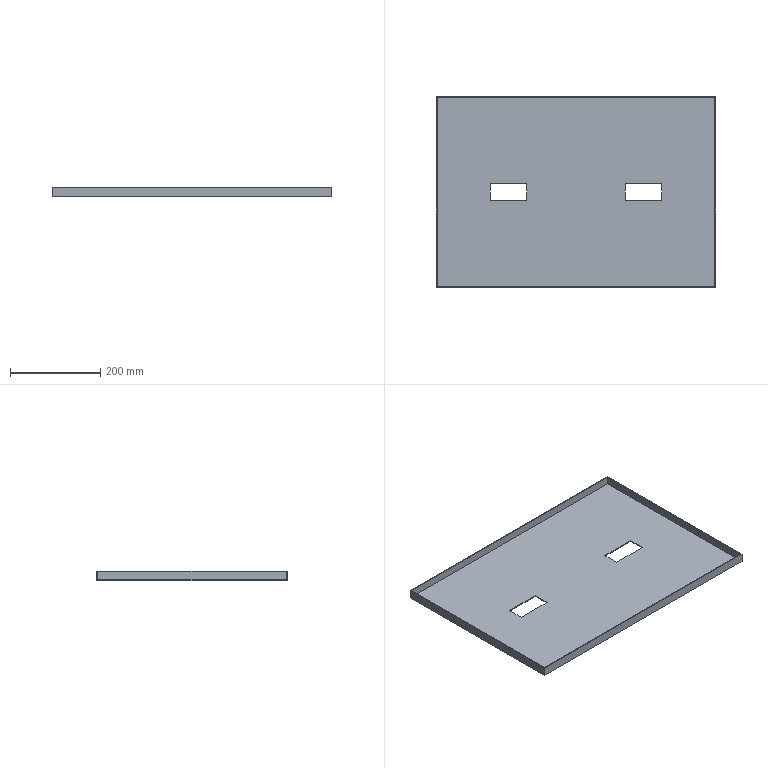Part | STEP file | Rear sealing plate | 1 solid | 19 faces | box 620 x 421.75 x 20 mm | volume 585700 mm3 | plane 19
STEP:
#1=CARTESIAN_POINT('',(0.,0.,0.));
#2=DIRECTION('',(0.,0.,1.));
#3=DIRECTION('',(1.,0.,0.));
#4=AXIS2_PLACEMENT_3D('',#1,#2,#3);
#5=CARTESIAN_POINT('',(-310.,-210.875,0.));
#6=VERTEX_POINT('',#5);
#7=CARTESIAN_POINT('',(310.,-210.875,0.));
#8=VERTEX_POINT('',#7);
#9=CARTESIAN_POINT('',(0.,-210.875,0.));
#10=DIRECTION('',(1.,0.,0.));
#11=VECTOR('',#10,1.);
#12=LINE('',#9,#11);
#13=CARTESIAN_POINT('',(0.,0.,0.));
#14=DIRECTION('',(0.,0.,1.));
#15=DIRECTION('',(1.,0.,0.));
#16=AXIS2_PLACEMENT_3D('',#13,#14,#15);
#17=PLANE('',#16);
#18=CARTESIAN_POINT('',(0.,-210.875));
#19=DIRECTION('',(1.,0.));
#20=VECTOR('',#19,1.);
#21=LINE('',#18,#20);
#22=(GEOMETRIC_REPRESENTATION_CONTEXT(2)PARAMETRIC_REPRESENTATION_CONTEXT()REPRESENTATION_CONTEXT('',''));
#23=DEFINITIONAL_REPRESENTATION('',(#21),#22);
#24=PCURVE('',#17,#23);
#25=CARTESIAN_POINT('',(-310.,-210.875,20.));
#26=DIRECTION('',(0.,1.,0.));
#27=DIRECTION('',(0.,0.,1.));
#28=AXIS2_PLACEMENT_3D('',#25,#26,#27);
#29=PLANE('',#28);
#30=CARTESIAN_POINT('',(-20.,310.));
#31=DIRECTION('',(0.,1.));
#32=VECTOR('',#31,1.);
#33=LINE('',#30,#32);
#34=(GEOMETRIC_REPRESENTATION_CONTEXT(2)PARAMETRIC_REPRESENTATION_CONTEXT()REPRESENTATION_CONTEXT('',''));
#35=DEFINITIONAL_REPRESENTATION('',(#33),#34);
#36=PCURVE('',#29,#35);
#37=SURFACE_CURVE('',#12,(#24,#36),.PCURVE_S1.);
#38=EDGE_CURVE('',#6,#8,#37,.T.);
#39=ORIENTED_EDGE('',*,*,#38,.F.);
#40=CARTESIAN_POINT('',(-310.,210.875,0.));
#41=VERTEX_POINT('',#40);
#42=CARTESIAN_POINT('',(-310.,0.,0.));
#43=DIRECTION('',(0.,-1.,0.));
#44=VECTOR('',#43,1.);
#45=LINE('',#42,#44);
#46=CARTESIAN_POINT('',(-310.,0.));
#47=DIRECTION('',(0.,-1.));
#48=VECTOR('',#47,1.);
#49=LINE('',#46,#48);
#50=(GEOMETRIC_REPRESENTATION_CONTEXT(2)PARAMETRIC_REPRESENTATION_CONTEXT()REPRESENTATION_CONTEXT('',''));
#51=DEFINITIONAL_REPRESENTATION('',(#49),#50);
#52=PCURVE('',#17,#51);
#53=CARTESIAN_POINT('',(-310.,210.875,20.));
#54=DIRECTION('',(1.,0.,0.));
#55=DIRECTION('',(0.,0.,-1.));
#56=AXIS2_PLACEMENT_3D('',#53,#54,#55);
#57=PLANE('',#56);
#58=CARTESIAN_POINT('',(20.,-210.875));
#59=DIRECTION('',(0.,-1.));
#60=VECTOR('',#59,1.);
#61=LINE('',#58,#60);
#62=(GEOMETRIC_REPRESENTATION_CONTEXT(2)PARAMETRIC_REPRESENTATION_CONTEXT()REPRESENTATION_CONTEXT('',''));
#63=DEFINITIONAL_REPRESENTATION('',(#61),#62);
#64=PCURVE('',#57,#63);
#65=SURFACE_CURVE('',#45,(#52,#64),.PCURVE_S1.);
#66=EDGE_CURVE('',#41,#6,#65,.T.);
#67=ORIENTED_EDGE('',*,*,#66,.F.);
#68=CARTESIAN_POINT('',(310.,210.875,0.));
#69=VERTEX_POINT('',#68);
#70=CARTESIAN_POINT('',(0.,210.875,0.));
#71=DIRECTION('',(-1.,0.,0.));
#72=VECTOR('',#71,1.);
#73=LINE('',#70,#72);
#74=CARTESIAN_POINT('',(0.,210.875));
#75=DIRECTION('',(-1.,0.));
#76=VECTOR('',#75,1.);
#77=LINE('',#74,#76);
#78=(GEOMETRIC_REPRESENTATION_CONTEXT(2)PARAMETRIC_REPRESENTATION_CONTEXT()REPRESENTATION_CONTEXT('',''));
#79=DEFINITIONAL_REPRESENTATION('',(#77),#78);
#80=PCURVE('',#17,#79);
#81=CARTESIAN_POINT('',(-310.,210.875,20.));
#82=DIRECTION('',(0.,-1.,0.));
#83=DIRECTION('',(0.,0.,-1.));
#84=AXIS2_PLACEMENT_3D('',#81,#82,#83);
#85=PLANE('',#84);
#86=CARTESIAN_POINT('',(20.,310.));
#87=DIRECTION('',(0.,-1.));
#88=VECTOR('',#87,1.);
#89=LINE('',#86,#88);
#90=(GEOMETRIC_REPRESENTATION_CONTEXT(2)PARAMETRIC_REPRESENTATION_CONTEXT()REPRESENTATION_CONTEXT('',''));
#91=DEFINITIONAL_REPRESENTATION('',(#89),#90);
#92=PCURVE('',#85,#91);
#93=SURFACE_CURVE('',#73,(#80,#92),.PCURVE_S1.);
#94=EDGE_CURVE('',#69,#41,#93,.T.);
#95=ORIENTED_EDGE('',*,*,#94,.F.);
#96=CARTESIAN_POINT('',(310.,0.,0.));
#97=DIRECTION('',(0.,1.,0.));
#98=VECTOR('',#97,1.);
#99=LINE('',#96,#98);
#100=CARTESIAN_POINT('',(310.,0.));
#101=DIRECTION('',(0.,1.));
#102=VECTOR('',#101,1.);
#103=LINE('',#100,#102);
#104=(GEOMETRIC_REPRESENTATION_CONTEXT(2)PARAMETRIC_REPRESENTATION_CONTEXT()REPRESENTATION_CONTEXT('',''));
#105=DEFINITIONAL_REPRESENTATION('',(#103),#104);
#106=PCURVE('',#17,#105);
#107=CARTESIAN_POINT('',(310.,210.875,20.));
#108=DIRECTION('',(-1.,0.,0.));
#109=DIRECTION('',(0.,-1.,0.));
#110=AXIS2_PLACEMENT_3D('',#107,#108,#109);
#111=PLANE('',#110);
#112=CARTESIAN_POINT('',(210.875,-20.));
#113=DIRECTION('',(-1.,0.));
#114=VECTOR('',#113,1.);
#115=LINE('',#112,#114);
#116=(GEOMETRIC_REPRESENTATION_CONTEXT(2)PARAMETRIC_REPRESENTATION_CONTEXT()REPRESENTATION_CONTEXT('',''));
#117=DEFINITIONAL_REPRESENTATION('',(#115),#116);
#118=PCURVE('',#111,#117);
#119=SURFACE_CURVE('',#99,(#106,#118),.PCURVE_S1.);
#120=EDGE_CURVE('',#8,#69,#119,.T.);
#121=ORIENTED_EDGE('',*,*,#120,.F.);
#122=EDGE_LOOP('',(#39,#67,#95,#121));
#123=FACE_BOUND('',#122,.T.);
#124=CARTESIAN_POINT('',(109.,-18.5,0.));
#125=VERTEX_POINT('',#124);
#126=CARTESIAN_POINT('',(109.,18.5,0.));
#127=VERTEX_POINT('',#126);
#128=CARTESIAN_POINT('',(109.,0.,0.));
#129=DIRECTION('',(0.,1.,0.));
#130=VECTOR('',#129,1.);
#131=LINE('',#128,#130);
#132=CARTESIAN_POINT('',(109.,0.));
#133=DIRECTION('',(0.,1.));
#134=VECTOR('',#133,1.);
#135=LINE('',#132,#134);
#136=(GEOMETRIC_REPRESENTATION_CONTEXT(2)PARAMETRIC_REPRESENTATION_CONTEXT()REPRESENTATION_CONTEXT('',''));
#137=DEFINITIONAL_REPRESENTATION('',(#135),#136);
#138=PCURVE('',#17,#137);
#139=CARTESIAN_POINT('',(109.,18.5,20.));
#140=DIRECTION('',(-1.,0.,0.));
#141=DIRECTION('',(0.,0.,1.));
#142=AXIS2_PLACEMENT_3D('',#139,#140,#141);
#143=PLANE('',#142);
#144=CARTESIAN_POINT('',(-20.,-18.5));
#145=DIRECTION('',(0.,1.));
#146=VECTOR('',#145,1.);
#147=LINE('',#144,#146);
#148=(GEOMETRIC_REPRESENTATION_CONTEXT(2)PARAMETRIC_REPRESENTATION_CONTEXT()REPRESENTATION_CONTEXT('',''));
#149=DEFINITIONAL_REPRESENTATION('',(#147),#148);
#150=PCURVE('',#143,#149);
#151=SURFACE_CURVE('',#131,(#138,#150),.PCURVE_S1.);
#152=EDGE_CURVE('',#125,#127,#151,.T.);
#153=ORIENTED_EDGE('',*,*,#152,.F.);
#154=CARTESIAN_POINT('',(190.,-18.5,0.));
#155=VERTEX_POINT('',#154);
#156=CARTESIAN_POINT('',(0.,-18.5,0.));
#157=DIRECTION('',(-1.,0.,0.));
#158=VECTOR('',#157,1.);
#159=LINE('',#156,#158);
#160=CARTESIAN_POINT('',(0.,-18.5));
#161=DIRECTION('',(-1.,0.));
#162=VECTOR('',#161,1.);
#163=LINE('',#160,#162);
#164=(GEOMETRIC_REPRESENTATION_CONTEXT(2)PARAMETRIC_REPRESENTATION_CONTEXT()REPRESENTATION_CONTEXT('',''));
#165=DEFINITIONAL_REPRESENTATION('',(#163),#164);
#166=PCURVE('',#17,#165);
#167=CARTESIAN_POINT('',(190.,-18.5,20.));
#168=DIRECTION('',(0.,-1.,0.));
#169=DIRECTION('',(0.,0.,-1.));
#170=AXIS2_PLACEMENT_3D('',#167,#168,#169);
#171=PLANE('',#170);
#172=CARTESIAN_POINT('',(20.,-190.));
#173=DIRECTION('',(0.,-1.));
#174=VECTOR('',#173,1.);
#175=LINE('',#172,#174);
#176=(GEOMETRIC_REPRESENTATION_CONTEXT(2)PARAMETRIC_REPRESENTATION_CONTEXT()REPRESENTATION_CONTEXT('',''));
#177=DEFINITIONAL_REPRESENTATION('',(#175),#176);
#178=PCURVE('',#171,#177);
#179=SURFACE_CURVE('',#159,(#166,#178),.PCURVE_S1.);
#180=EDGE_CURVE('',#155,#125,#179,.T.);
#181=ORIENTED_EDGE('',*,*,#180,.F.);
#182=CARTESIAN_POINT('',(190.,18.5,0.));
#183=VERTEX_POINT('',#182);
#184=CARTESIAN_POINT('',(190.,0.,0.));
#185=DIRECTION('',(0.,-1.,0.));
#186=VECTOR('',#185,1.);
#187=LINE('',#184,#186);
#188=CARTESIAN_POINT('',(190.,0.));
#189=DIRECTION('',(0.,-1.));
#190=VECTOR('',#189,1.);
#191=LINE('',#188,#190);
#192=(GEOMETRIC_REPRESENTATION_CONTEXT(2)PARAMETRIC_REPRESENTATION_CONTEXT()REPRESENTATION_CONTEXT('',''));
#193=DEFINITIONAL_REPRESENTATION('',(#191),#192);
#194=PCURVE('',#17,#193);
#195=CARTESIAN_POINT('',(190.,18.5,20.));
#196=DIRECTION('',(1.,0.,0.));
#197=DIRECTION('',(0.,0.,-1.));
#198=AXIS2_PLACEMENT_3D('',#195,#196,#197);
#199=PLANE('',#198);
#200=CARTESIAN_POINT('',(20.,-18.5));
#201=DIRECTION('',(0.,-1.));
#202=VECTOR('',#201,1.);
#203=LINE('',#200,#202);
#204=(GEOMETRIC_REPRESENTATION_CONTEXT(2)PARAMETRIC_REPRESENTATION_CONTEXT()REPRESENTATION_CONTEXT('',''));
#205=DEFINITIONAL_REPRESENTATION('',(#203),#204);
#206=PCURVE('',#199,#205);
#207=SURFACE_CURVE('',#187,(#194,#206),.PCURVE_S1.);
#208=EDGE_CURVE('',#183,#155,#207,.T.);
#209=ORIENTED_EDGE('',*,*,#208,.F.);
#210=CARTESIAN_POINT('',(0.,18.5,0.));
#211=DIRECTION('',(1.,0.,0.));
#212=VECTOR('',#211,1.);
#213=LINE('',#210,#212);
#214=CARTESIAN_POINT('',(0.,18.5));
#215=DIRECTION('',(1.,0.));
#216=VECTOR('',#215,1.);
#217=LINE('',#214,#216);
#218=(GEOMETRIC_REPRESENTATION_CONTEXT(2)PARAMETRIC_REPRESENTATION_CONTEXT()REPRESENTATION_CONTEXT('',''));
#219=DEFINITIONAL_REPRESENTATION('',(#217),#218);
#220=PCURVE('',#17,#219);
#221=CARTESIAN_POINT('',(190.,18.5,20.));
#222=DIRECTION('',(0.,1.,0.));
#223=DIRECTION('',(-1.,0.,0.));
#224=AXIS2_PLACEMENT_3D('',#221,#222,#223);
#225=PLANE('',#224);
#226=CARTESIAN_POINT('',(190.,-20.));
#227=DIRECTION('',(-1.,0.));
#228=VECTOR('',#227,1.);
#229=LINE('',#226,#228);
#230=(GEOMETRIC_REPRESENTATION_CONTEXT(2)PARAMETRIC_REPRESENTATION_CONTEXT()REPRESENTATION_CONTEXT('',''));
#231=DEFINITIONAL_REPRESENTATION('',(#229),#230);
#232=PCURVE('',#225,#231);
#233=SURFACE_CURVE('',#213,(#220,#232),.PCURVE_S1.);
#234=EDGE_CURVE('',#127,#183,#233,.T.);
#235=ORIENTED_EDGE('',*,*,#234,.F.);
#236=EDGE_LOOP('',(#153,#181,#209,#235));
#237=FACE_BOUND('',#236,.T.);
#238=CARTESIAN_POINT('',(-190.,-18.5,0.));
#239=VERTEX_POINT('',#238);
#240=CARTESIAN_POINT('',(-190.,18.5,0.));
#241=VERTEX_POINT('',#240);
#242=CARTESIAN_POINT('',(-190.,0.,0.));
#243=DIRECTION('',(0.,1.,0.));
#244=VECTOR('',#243,1.);
#245=LINE('',#242,#244);
#246=CARTESIAN_POINT('',(-190.,0.));
#247=DIRECTION('',(0.,1.));
#248=VECTOR('',#247,1.);
#249=LINE('',#246,#248);
#250=(GEOMETRIC_REPRESENTATION_CONTEXT(2)PARAMETRIC_REPRESENTATION_CONTEXT()REPRESENTATION_CONTEXT('',''));
#251=DEFINITIONAL_REPRESENTATION('',(#249),#250);
#252=PCURVE('',#17,#251);
#253=CARTESIAN_POINT('',(-190.,18.5,20.));
#254=DIRECTION('',(-1.,0.,0.));
#255=DIRECTION('',(0.,0.,1.));
#256=AXIS2_PLACEMENT_3D('',#253,#254,#255);
#257=PLANE('',#256);
#258=CARTESIAN_POINT('',(-20.,-18.5));
#259=DIRECTION('',(0.,1.));
#260=VECTOR('',#259,1.);
#261=LINE('',#258,#260);
#262=(GEOMETRIC_REPRESENTATION_CONTEXT(2)PARAMETRIC_REPRESENTATION_CONTEXT()REPRESENTATION_CONTEXT('',''));
#263=DEFINITIONAL_REPRESENTATION('',(#261),#262);
#264=PCURVE('',#257,#263);
#265=SURFACE_CURVE('',#245,(#252,#264),.PCURVE_S1.);
#266=EDGE_CURVE('',#239,#241,#265,.T.);
#267=ORIENTED_EDGE('',*,*,#266,.F.);
#268=CARTESIAN_POINT('',(-109.,-18.5,0.));
#269=VERTEX_POINT('',#268);
#270=CARTESIAN_POINT('',(0.,-18.5,0.));
#271=DIRECTION('',(-1.,0.,0.));
#272=VECTOR('',#271,1.);
#273=LINE('',#270,#272);
#274=CARTESIAN_POINT('',(0.,-18.5));
#275=DIRECTION('',(-1.,0.));
#276=VECTOR('',#275,1.);
#277=LINE('',#274,#276);
#278=(GEOMETRIC_REPRESENTATION_CONTEXT(2)PARAMETRIC_REPRESENTATION_CONTEXT()REPRESENTATION_CONTEXT('',''));
#279=DEFINITIONAL_REPRESENTATION('',(#277),#278);
#280=PCURVE('',#17,#279);
#281=CARTESIAN_POINT('',(-109.,-18.5,20.));
#282=DIRECTION('',(0.,-1.,0.));
#283=DIRECTION('',(0.,0.,-1.));
#284=AXIS2_PLACEMENT_3D('',#281,#282,#283);
#285=PLANE('',#284);
#286=CARTESIAN_POINT('',(20.,109.));
#287=DIRECTION('',(0.,-1.));
#288=VECTOR('',#287,1.);
#289=LINE('',#286,#288);
#290=(GEOMETRIC_REPRESENTATION_CONTEXT(2)PARAMETRIC_REPRESENTATION_CONTEXT()REPRESENTATION_CONTEXT('',''));
#291=DEFINITIONAL_REPRESENTATION('',(#289),#290);
#292=PCURVE('',#285,#291);
#293=SURFACE_CURVE('',#273,(#280,#292),.PCURVE_S1.);
#294=EDGE_CURVE('',#269,#239,#293,.T.);
#295=ORIENTED_EDGE('',*,*,#294,.F.);
#296=CARTESIAN_POINT('',(-109.,18.5,0.));
#297=VERTEX_POINT('',#296);
#298=CARTESIAN_POINT('',(-109.,0.,0.));
#299=DIRECTION('',(0.,-1.,0.));
#300=VECTOR('',#299,1.);
#301=LINE('',#298,#300);
#302=CARTESIAN_POINT('',(-109.,0.));
#303=DIRECTION('',(0.,-1.));
#304=VECTOR('',#303,1.);
#305=LINE('',#302,#304);
#306=(GEOMETRIC_REPRESENTATION_CONTEXT(2)PARAMETRIC_REPRESENTATION_CONTEXT()REPRESENTATION_CONTEXT('',''));
#307=DEFINITIONAL_REPRESENTATION('',(#305),#306);
#308=PCURVE('',#17,#307);
#309=CARTESIAN_POINT('',(-109.,18.5,20.));
#310=DIRECTION('',(1.,0.,0.));
#311=DIRECTION('',(0.,1.,0.));
#312=AXIS2_PLACEMENT_3D('',#309,#310,#311);
#313=PLANE('',#312);
#314=CARTESIAN_POINT('',(-18.5,-20.));
#315=DIRECTION('',(-1.,0.));
#316=VECTOR('',#315,1.);
#317=LINE('',#314,#316);
#318=(GEOMETRIC_REPRESENTATION_CONTEXT(2)PARAMETRIC_REPRESENTATION_CONTEXT()REPRESENTATION_CONTEXT('',''));
#319=DEFINITIONAL_REPRESENTATION('',(#317),#318);
#320=PCURVE('',#313,#319);
#321=SURFACE_CURVE('',#301,(#308,#320),.PCURVE_S1.);
#322=EDGE_CURVE('',#297,#269,#321,.T.);
#323=ORIENTED_EDGE('',*,*,#322,.F.);
#324=CARTESIAN_POINT('',(0.,18.5,0.));
#325=DIRECTION('',(1.,0.,0.));
#326=VECTOR('',#325,1.);
#327=LINE('',#324,#326);
#328=CARTESIAN_POINT('',(0.,18.5));
#329=DIRECTION('',(1.,0.));
#330=VECTOR('',#329,1.);
#331=LINE('',#328,#330);
#332=(GEOMETRIC_REPRESENTATION_CONTEXT(2)PARAMETRIC_REPRESENTATION_CONTEXT()REPRESENTATION_CONTEXT('',''));
#333=DEFINITIONAL_REPRESENTATION('',(#331),#332);
#334=PCURVE('',#17,#333);
#335=CARTESIAN_POINT('',(-109.,18.5,20.));
#336=DIRECTION('',(0.,1.,0.));
#337=DIRECTION('',(0.,0.,1.));
#338=AXIS2_PLACEMENT_3D('',#335,#336,#337);
#339=PLANE('',#338);
#340=CARTESIAN_POINT('',(-20.,109.));
#341=DIRECTION('',(0.,1.));
#342=VECTOR('',#341,1.);
#343=LINE('',#340,#342);
#344=(GEOMETRIC_REPRESENTATION_CONTEXT(2)PARAMETRIC_REPRESENTATION_CONTEXT()REPRESENTATION_CONTEXT('',''));
#345=DEFINITIONAL_REPRESENTATION('',(#343),#344);
#346=PCURVE('',#339,#345);
#347=SURFACE_CURVE('',#327,(#334,#346),.PCURVE_S1.);
#348=EDGE_CURVE('',#241,#297,#347,.T.);
#349=ORIENTED_EDGE('',*,*,#348,.F.);
#350=EDGE_LOOP('',(#267,#295,#323,#349));
#351=FACE_BOUND('',#350,.T.);
#352=ADVANCED_FACE('',(#123,#237,#351),#17,.F.);
#353=CARTESIAN_POINT('',(310.,210.875,20.));
#354=VERTEX_POINT('',#353);
#355=CARTESIAN_POINT('',(310.,210.875,20.));
#356=DIRECTION('',(0.,0.,-1.));
#357=VECTOR('',#356,1.);
#358=LINE('',#355,#357);
#359=CARTESIAN_POINT('',(0.,0.));
#360=DIRECTION('',(0.,-1.));
#361=VECTOR('',#360,1.);
#362=LINE('',#359,#361);
#363=(GEOMETRIC_REPRESENTATION_CONTEXT(2)PARAMETRIC_REPRESENTATION_CONTEXT()REPRESENTATION_CONTEXT('',''));
#364=DEFINITIONAL_REPRESENTATION('',(#362),#363);
#365=PCURVE('',#111,#364);
#366=CARTESIAN_POINT('',(0.,620.));
#367=DIRECTION('',(1.,0.));
#368=VECTOR('',#367,1.);
#369=LINE('',#366,#368);
#370=(GEOMETRIC_REPRESENTATION_CONTEXT(2)PARAMETRIC_REPRESENTATION_CONTEXT()REPRESENTATION_CONTEXT('',''));
#371=DEFINITIONAL_REPRESENTATION('',(#369),#370);
#372=PCURVE('',#85,#371);
#373=SURFACE_CURVE('',#358,(#365,#372),.PCURVE_S1.);
#374=EDGE_CURVE('',#354,#69,#373,.T.);
#375=ORIENTED_EDGE('',*,*,#374,.F.);
#376=CARTESIAN_POINT('',(310.,-210.875,20.));
#377=VERTEX_POINT('',#376);
#378=CARTESIAN_POINT('',(310.,210.875,20.));
#379=DIRECTION('',(0.,1.,0.));
#380=VECTOR('',#379,1.);
#381=LINE('',#378,#380);
#382=CARTESIAN_POINT('',(0.,0.));
#383=DIRECTION('',(-1.,0.));
#384=VECTOR('',#383,1.);
#385=LINE('',#382,#384);
#386=(GEOMETRIC_REPRESENTATION_CONTEXT(2)PARAMETRIC_REPRESENTATION_CONTEXT()REPRESENTATION_CONTEXT('',''));
#387=DEFINITIONAL_REPRESENTATION('',(#385),#386);
#388=PCURVE('',#111,#387);
#389=CARTESIAN_POINT('',(0.,0.,20.));
#390=DIRECTION('',(0.,0.,1.));
#391=DIRECTION('',(1.,0.,0.));
#392=AXIS2_PLACEMENT_3D('',#389,#390,#391);
#393=PLANE('',#392);
#394=CARTESIAN_POINT('',(310.,210.875));
#395=DIRECTION('',(0.,1.));
#396=VECTOR('',#395,1.);
#397=LINE('',#394,#396);
#398=(GEOMETRIC_REPRESENTATION_CONTEXT(2)PARAMETRIC_REPRESENTATION_CONTEXT()REPRESENTATION_CONTEXT('',''));
#399=DEFINITIONAL_REPRESENTATION('',(#397),#398);
#400=PCURVE('',#393,#399);
#401=SURFACE_CURVE('',#381,(#388,#400),.PCURVE_S1.);
#402=EDGE_CURVE('',#377,#354,#401,.T.);
#403=ORIENTED_EDGE('',*,*,#402,.F.);
#404=CARTESIAN_POINT('',(310.,-210.875,20.));
#405=DIRECTION('',(0.,0.,1.));
#406=VECTOR('',#405,1.);
#407=LINE('',#404,#406);
#408=CARTESIAN_POINT('',(421.75,0.));
#409=DIRECTION('',(0.,1.));
#410=VECTOR('',#409,1.);
#411=LINE('',#408,#410);
#412=(GEOMETRIC_REPRESENTATION_CONTEXT(2)PARAMETRIC_REPRESENTATION_CONTEXT()REPRESENTATION_CONTEXT('',''));
#413=DEFINITIONAL_REPRESENTATION('',(#411),#412);
#414=PCURVE('',#111,#413);
#415=CARTESIAN_POINT('',(0.,620.));
#416=DIRECTION('',(1.,0.));
#417=VECTOR('',#416,1.);
#418=LINE('',#415,#417);
#419=(GEOMETRIC_REPRESENTATION_CONTEXT(2)PARAMETRIC_REPRESENTATION_CONTEXT()REPRESENTATION_CONTEXT('',''));
#420=DEFINITIONAL_REPRESENTATION('',(#418),#419);
#421=PCURVE('',#29,#420);
#422=SURFACE_CURVE('',#407,(#414,#421),.PCURVE_S1.);
#423=EDGE_CURVE('',#8,#377,#422,.T.);
#424=ORIENTED_EDGE('',*,*,#423,.F.);
#425=ORIENTED_EDGE('',*,*,#120,.T.);
#426=EDGE_LOOP('',(#375,#403,#424,#425));
#427=FACE_BOUND('',#426,.T.);
#428=ADVANCED_FACE('',(#427),#111,.F.);
#429=ORIENTED_EDGE('',*,*,#423,.T.);
#430=CARTESIAN_POINT('',(-310.,-210.875,20.));
#431=VERTEX_POINT('',#430);
#432=CARTESIAN_POINT('',(-310.,-210.875,20.));
#433=DIRECTION('',(1.,0.,0.));
#434=VECTOR('',#433,1.);
#435=LINE('',#432,#434);
#436=CARTESIAN_POINT('',(0.,0.));
#437=DIRECTION('',(0.,1.));
#438=VECTOR('',#437,1.);
#439=LINE('',#436,#438);
#440=(GEOMETRIC_REPRESENTATION_CONTEXT(2)PARAMETRIC_REPRESENTATION_CONTEXT()REPRESENTATION_CONTEXT('',''));
#441=DEFINITIONAL_REPRESENTATION('',(#439),#440);
#442=PCURVE('',#29,#441);
#443=CARTESIAN_POINT('',(-310.,-210.875));
#444=DIRECTION('',(1.,0.));
#445=VECTOR('',#444,1.);
#446=LINE('',#443,#445);
#447=(GEOMETRIC_REPRESENTATION_CONTEXT(2)PARAMETRIC_REPRESENTATION_CONTEXT()REPRESENTATION_CONTEXT('',''));
#448=DEFINITIONAL_REPRESENTATION('',(#446),#447);
#449=PCURVE('',#393,#448);
#450=SURFACE_CURVE('',#435,(#442,#449),.PCURVE_S1.);
#451=EDGE_CURVE('',#431,#377,#450,.T.);
#452=ORIENTED_EDGE('',*,*,#451,.F.);
#453=CARTESIAN_POINT('',(-310.,-210.875,20.));
#454=DIRECTION('',(0.,0.,1.));
#455=VECTOR('',#454,1.);
#456=LINE('',#453,#455);
#457=CARTESIAN_POINT('',(0.,0.));
#458=DIRECTION('',(1.,0.));
#459=VECTOR('',#458,1.);
#460=LINE('',#457,#459);
#461=(GEOMETRIC_REPRESENTATION_CONTEXT(2)PARAMETRIC_REPRESENTATION_CONTEXT()REPRESENTATION_CONTEXT('',''));
#462=DEFINITIONAL_REPRESENTATION('',(#460),#461);
#463=PCURVE('',#29,#462);
#464=CARTESIAN_POINT('',(0.,-421.75));
#465=DIRECTION('',(-1.,0.));
#466=VECTOR('',#465,1.);
#467=LINE('',#464,#466);
#468=(GEOMETRIC_REPRESENTATION_CONTEXT(2)PARAMETRIC_REPRESENTATION_CONTEXT()REPRESENTATION_CONTEXT('',''));
#469=DEFINITIONAL_REPRESENTATION('',(#467),#468);
#470=PCURVE('',#57,#469);
#471=SURFACE_CURVE('',#456,(#463,#470),.PCURVE_S1.);
#472=EDGE_CURVE('',#6,#431,#471,.T.);
#473=ORIENTED_EDGE('',*,*,#472,.F.);
#474=ORIENTED_EDGE('',*,*,#38,.T.);
#475=EDGE_LOOP('',(#429,#452,#473,#474));
#476=FACE_BOUND('',#475,.T.);
#477=ADVANCED_FACE('',(#476),#29,.F.);
#478=ORIENTED_EDGE('',*,*,#472,.T.);
#479=CARTESIAN_POINT('',(-310.,210.875,20.));
#480=VERTEX_POINT('',#479);
#481=CARTESIAN_POINT('',(-310.,210.875,20.));
#482=DIRECTION('',(0.,-1.,0.));
#483=VECTOR('',#482,1.);
#484=LINE('',#481,#483);
#485=CARTESIAN_POINT('',(0.,0.));
#486=DIRECTION('',(0.,-1.));
#487=VECTOR('',#486,1.);
#488=LINE('',#485,#487);
#489=(GEOMETRIC_REPRESENTATION_CONTEXT(2)PARAMETRIC_REPRESENTATION_CONTEXT()REPRESENTATION_CONTEXT('',''));
#490=DEFINITIONAL_REPRESENTATION('',(#488),#489);
#491=PCURVE('',#57,#490);
#492=CARTESIAN_POINT('',(-310.,210.875));
#493=DIRECTION('',(0.,-1.));
#494=VECTOR('',#493,1.);
#495=LINE('',#492,#494);
#496=(GEOMETRIC_REPRESENTATION_CONTEXT(2)PARAMETRIC_REPRESENTATION_CONTEXT()REPRESENTATION_CONTEXT('',''));
#497=DEFINITIONAL_REPRESENTATION('',(#495),#496);
#498=PCURVE('',#393,#497);
#499=SURFACE_CURVE('',#484,(#491,#498),.PCURVE_S1.);
#500=EDGE_CURVE('',#480,#431,#499,.T.);
#501=ORIENTED_EDGE('',*,*,#500,.F.);
#502=CARTESIAN_POINT('',(-310.,210.875,20.));
#503=DIRECTION('',(0.,0.,1.));
#504=VECTOR('',#503,1.);
#505=LINE('',#502,#504);
#506=CARTESIAN_POINT('',(0.,0.));
#507=DIRECTION('',(-1.,0.));
#508=VECTOR('',#507,1.);
#509=LINE('',#506,#508);
#510=(GEOMETRIC_REPRESENTATION_CONTEXT(2)PARAMETRIC_REPRESENTATION_CONTEXT()REPRESENTATION_CONTEXT('',''));
#511=DEFINITIONAL_REPRESENTATION('',(#509),#510);
#512=PCURVE('',#57,#511);
#513=CARTESIAN_POINT('',(0.,0.));
#514=DIRECTION('',(-1.,0.));
#515=VECTOR('',#514,1.);
#516=LINE('',#513,#515);
#517=(GEOMETRIC_REPRESENTATION_CONTEXT(2)PARAMETRIC_REPRESENTATION_CONTEXT()REPRESENTATION_CONTEXT('',''));
#518=DEFINITIONAL_REPRESENTATION('',(#516),#517);
#519=PCURVE('',#85,#518);
#520=SURFACE_CURVE('',#505,(#512,#519),.PCURVE_S1.);
#521=EDGE_CURVE('',#41,#480,#520,.T.);
#522=ORIENTED_EDGE('',*,*,#521,.F.);
#523=ORIENTED_EDGE('',*,*,#66,.T.);
#524=EDGE_LOOP('',(#478,#501,#522,#523));
#525=FACE_BOUND('',#524,.T.);
#526=ADVANCED_FACE('',(#525),#57,.F.);
#527=ORIENTED_EDGE('',*,*,#521,.T.);
#528=CARTESIAN_POINT('',(-310.,210.875,20.));
#529=DIRECTION('',(-1.,0.,0.));
#530=VECTOR('',#529,1.);
#531=LINE('',#528,#530);
#532=CARTESIAN_POINT('',(0.,0.));
#533=DIRECTION('',(0.,-1.));
#534=VECTOR('',#533,1.);
#535=LINE('',#532,#534);
#536=(GEOMETRIC_REPRESENTATION_CONTEXT(2)PARAMETRIC_REPRESENTATION_CONTEXT()REPRESENTATION_CONTEXT('',''));
#537=DEFINITIONAL_REPRESENTATION('',(#535),#536);
#538=PCURVE('',#85,#537);
#539=CARTESIAN_POINT('',(-310.,210.875));
#540=DIRECTION('',(-1.,0.));
#541=VECTOR('',#540,1.);
#542=LINE('',#539,#541);
#543=(GEOMETRIC_REPRESENTATION_CONTEXT(2)PARAMETRIC_REPRESENTATION_CONTEXT()REPRESENTATION_CONTEXT('',''));
#544=DEFINITIONAL_REPRESENTATION('',(#542),#543);
#545=PCURVE('',#393,#544);
#546=SURFACE_CURVE('',#531,(#538,#545),.PCURVE_S1.);
#547=EDGE_CURVE('',#354,#480,#546,.T.);
#548=ORIENTED_EDGE('',*,*,#547,.F.);
#549=ORIENTED_EDGE('',*,*,#374,.T.);
#550=ORIENTED_EDGE('',*,*,#94,.T.);
#551=EDGE_LOOP('',(#527,#548,#549,#550));
#552=FACE_BOUND('',#551,.T.);
#553=ADVANCED_FACE('',(#552),#85,.F.);
#554=CARTESIAN_POINT('',(109.,18.5,2.));
#555=VERTEX_POINT('',#554);
#556=CARTESIAN_POINT('',(109.,18.5,20.));
#557=DIRECTION('',(0.,0.,1.));
#558=VECTOR('',#557,1.);
#559=LINE('',#556,#558);
#560=CARTESIAN_POINT('',(81.,0.));
#561=DIRECTION('',(0.,1.));
#562=VECTOR('',#561,1.);
#563=LINE('',#560,#562);
#564=(GEOMETRIC_REPRESENTATION_CONTEXT(2)PARAMETRIC_REPRESENTATION_CONTEXT()REPRESENTATION_CONTEXT('',''));
#565=DEFINITIONAL_REPRESENTATION('',(#563),#564);
#566=PCURVE('',#225,#565);
#567=CARTESIAN_POINT('',(0.,0.));
#568=DIRECTION('',(1.,0.));
#569=VECTOR('',#568,1.);
#570=LINE('',#567,#569);
#571=(GEOMETRIC_REPRESENTATION_CONTEXT(2)PARAMETRIC_REPRESENTATION_CONTEXT()REPRESENTATION_CONTEXT('',''));
#572=DEFINITIONAL_REPRESENTATION('',(#570),#571);
#573=PCURVE('',#143,#572);
#574=SURFACE_CURVE('',#559,(#566,#573),.PCURVE_S1.);
#575=EDGE_CURVE('',#127,#555,#574,.T.);
#576=ORIENTED_EDGE('',*,*,#575,.F.);
#577=ORIENTED_EDGE('',*,*,#234,.T.);
#578=CARTESIAN_POINT('',(190.,18.5,2.));
#579=VERTEX_POINT('',#578);
#580=CARTESIAN_POINT('',(190.,18.5,20.));
#581=DIRECTION('',(0.,0.,-1.));
#582=VECTOR('',#581,1.);
#583=LINE('',#580,#582);
#584=CARTESIAN_POINT('',(0.,0.));
#585=DIRECTION('',(0.,-1.));
#586=VECTOR('',#585,1.);
#587=LINE('',#584,#586);
#588=(GEOMETRIC_REPRESENTATION_CONTEXT(2)PARAMETRIC_REPRESENTATION_CONTEXT()REPRESENTATION_CONTEXT('',''));
#589=DEFINITIONAL_REPRESENTATION('',(#587),#588);
#590=PCURVE('',#225,#589);
#591=CARTESIAN_POINT('',(0.,0.));
#592=DIRECTION('',(1.,0.));
#593=VECTOR('',#592,1.);
#594=LINE('',#591,#593);
#595=(GEOMETRIC_REPRESENTATION_CONTEXT(2)PARAMETRIC_REPRESENTATION_CONTEXT()REPRESENTATION_CONTEXT('',''));
#596=DEFINITIONAL_REPRESENTATION('',(#594),#595);
#597=PCURVE('',#199,#596);
#598=SURFACE_CURVE('',#583,(#590,#597),.PCURVE_S1.);
#599=EDGE_CURVE('',#579,#183,#598,.T.);
#600=ORIENTED_EDGE('',*,*,#599,.F.);
#601=CARTESIAN_POINT('',(190.,18.5,2.));
#602=DIRECTION('',(1.,0.,0.));
#603=VECTOR('',#602,1.);
#604=LINE('',#601,#603);
#605=CARTESIAN_POINT('',(0.,-18.));
#606=DIRECTION('',(-1.,0.));
#607=VECTOR('',#606,1.);
#608=LINE('',#605,#607);
#609=(GEOMETRIC_REPRESENTATION_CONTEXT(2)PARAMETRIC_REPRESENTATION_CONTEXT()REPRESENTATION_CONTEXT('',''));
#610=DEFINITIONAL_REPRESENTATION('',(#608),#609);
#611=PCURVE('',#225,#610);
#612=CARTESIAN_POINT('',(0.,0.,2.));
#613=DIRECTION('',(0.,0.,1.));
#614=DIRECTION('',(1.,0.,0.));
#615=AXIS2_PLACEMENT_3D('',#612,#613,#614);
#616=PLANE('',#615);
#617=CARTESIAN_POINT('',(190.,18.5));
#618=DIRECTION('',(1.,0.));
#619=VECTOR('',#618,1.);
#620=LINE('',#617,#619);
#621=(GEOMETRIC_REPRESENTATION_CONTEXT(2)PARAMETRIC_REPRESENTATION_CONTEXT()REPRESENTATION_CONTEXT('',''));
#622=DEFINITIONAL_REPRESENTATION('',(#620),#621);
#623=PCURVE('',#616,#622);
#624=SURFACE_CURVE('',#604,(#611,#623),.PCURVE_S1.);
#625=EDGE_CURVE('',#555,#579,#624,.T.);
#626=ORIENTED_EDGE('',*,*,#625,.F.);
#627=EDGE_LOOP('',(#576,#577,#600,#626));
#628=FACE_BOUND('',#627,.T.);
#629=ADVANCED_FACE('',(#628),#225,.F.);
#630=CARTESIAN_POINT('',(109.,-18.5,2.));
#631=VERTEX_POINT('',#630);
#632=CARTESIAN_POINT('',(109.,-18.5,20.));
#633=DIRECTION('',(0.,0.,1.));
#634=VECTOR('',#633,1.);
#635=LINE('',#632,#634);
#636=CARTESIAN_POINT('',(0.,-37.));
#637=DIRECTION('',(1.,0.));
#638=VECTOR('',#637,1.);
#639=LINE('',#636,#638);
#640=(GEOMETRIC_REPRESENTATION_CONTEXT(2)PARAMETRIC_REPRESENTATION_CONTEXT()REPRESENTATION_CONTEXT('',''));
#641=DEFINITIONAL_REPRESENTATION('',(#639),#640);
#642=PCURVE('',#143,#641);
#643=CARTESIAN_POINT('',(0.,-81.));
#644=DIRECTION('',(-1.,0.));
#645=VECTOR('',#644,1.);
#646=LINE('',#643,#645);
#647=(GEOMETRIC_REPRESENTATION_CONTEXT(2)PARAMETRIC_REPRESENTATION_CONTEXT()REPRESENTATION_CONTEXT('',''));
#648=DEFINITIONAL_REPRESENTATION('',(#646),#647);
#649=PCURVE('',#171,#648);
#650=SURFACE_CURVE('',#635,(#642,#649),.PCURVE_S1.);
#651=EDGE_CURVE('',#125,#631,#650,.T.);
#652=ORIENTED_EDGE('',*,*,#651,.F.);
#653=ORIENTED_EDGE('',*,*,#152,.T.);
#654=ORIENTED_EDGE('',*,*,#575,.T.);
#655=CARTESIAN_POINT('',(109.,18.5,2.));
#656=DIRECTION('',(0.,1.,0.));
#657=VECTOR('',#656,1.);
#658=LINE('',#655,#657);
#659=CARTESIAN_POINT('',(-18.,0.));
#660=DIRECTION('',(0.,1.));
#661=VECTOR('',#660,1.);
#662=LINE('',#659,#661);
#663=(GEOMETRIC_REPRESENTATION_CONTEXT(2)PARAMETRIC_REPRESENTATION_CONTEXT()REPRESENTATION_CONTEXT('',''));
#664=DEFINITIONAL_REPRESENTATION('',(#662),#663);
#665=PCURVE('',#143,#664);
#666=CARTESIAN_POINT('',(109.,18.5));
#667=DIRECTION('',(0.,1.));
#668=VECTOR('',#667,1.);
#669=LINE('',#666,#668);
#670=(GEOMETRIC_REPRESENTATION_CONTEXT(2)PARAMETRIC_REPRESENTATION_CONTEXT()REPRESENTATION_CONTEXT('',''));
#671=DEFINITIONAL_REPRESENTATION('',(#669),#670);
#672=PCURVE('',#616,#671);
#673=SURFACE_CURVE('',#658,(#665,#672),.PCURVE_S1.);
#674=EDGE_CURVE('',#631,#555,#673,.T.);
#675=ORIENTED_EDGE('',*,*,#674,.F.);
#676=EDGE_LOOP('',(#652,#653,#654,#675));
#677=FACE_BOUND('',#676,.T.);
#678=ADVANCED_FACE('',(#677),#143,.F.);
#679=CARTESIAN_POINT('',(190.,-18.5,2.));
#680=VERTEX_POINT('',#679);
#681=CARTESIAN_POINT('',(190.,-18.5,20.));
#682=DIRECTION('',(0.,0.,1.));
#683=VECTOR('',#682,1.);
#684=LINE('',#681,#683);
#685=CARTESIAN_POINT('',(0.,0.));
#686=DIRECTION('',(-1.,0.));
#687=VECTOR('',#686,1.);
#688=LINE('',#685,#687);
#689=(GEOMETRIC_REPRESENTATION_CONTEXT(2)PARAMETRIC_REPRESENTATION_CONTEXT()REPRESENTATION_CONTEXT('',''));
#690=DEFINITIONAL_REPRESENTATION('',(#688),#689);
#691=PCURVE('',#171,#690);
#692=CARTESIAN_POINT('',(0.,-37.));
#693=DIRECTION('',(-1.,0.));
#694=VECTOR('',#693,1.);
#695=LINE('',#692,#694);
#696=(GEOMETRIC_REPRESENTATION_CONTEXT(2)PARAMETRIC_REPRESENTATION_CONTEXT()REPRESENTATION_CONTEXT('',''));
#697=DEFINITIONAL_REPRESENTATION('',(#695),#696);
#698=PCURVE('',#199,#697);
#699=SURFACE_CURVE('',#684,(#691,#698),.PCURVE_S1.);
#700=EDGE_CURVE('',#155,#680,#699,.T.);
#701=ORIENTED_EDGE('',*,*,#700,.F.);
#702=ORIENTED_EDGE('',*,*,#180,.T.);
#703=ORIENTED_EDGE('',*,*,#651,.T.);
#704=CARTESIAN_POINT('',(190.,-18.5,2.));
#705=DIRECTION('',(-1.,0.,0.));
#706=VECTOR('',#705,1.);
#707=LINE('',#704,#706);
#708=CARTESIAN_POINT('',(18.,0.));
#709=DIRECTION('',(0.,-1.));
#710=VECTOR('',#709,1.);
#711=LINE('',#708,#710);
#712=(GEOMETRIC_REPRESENTATION_CONTEXT(2)PARAMETRIC_REPRESENTATION_CONTEXT()REPRESENTATION_CONTEXT('',''));
#713=DEFINITIONAL_REPRESENTATION('',(#711),#712);
#714=PCURVE('',#171,#713);
#715=CARTESIAN_POINT('',(190.,-18.5));
#716=DIRECTION('',(-1.,0.));
#717=VECTOR('',#716,1.);
#718=LINE('',#715,#717);
#719=(GEOMETRIC_REPRESENTATION_CONTEXT(2)PARAMETRIC_REPRESENTATION_CONTEXT()REPRESENTATION_CONTEXT('',''));
#720=DEFINITIONAL_REPRESENTATION('',(#718),#719);
#721=PCURVE('',#616,#720);
#722=SURFACE_CURVE('',#707,(#714,#721),.PCURVE_S1.);
#723=EDGE_CURVE('',#680,#631,#722,.T.);
#724=ORIENTED_EDGE('',*,*,#723,.F.);
#725=EDGE_LOOP('',(#701,#702,#703,#724));
#726=FACE_BOUND('',#725,.T.);
#727=ADVANCED_FACE('',(#726),#171,.F.);
#728=ORIENTED_EDGE('',*,*,#599,.T.);
#729=ORIENTED_EDGE('',*,*,#208,.T.);
#730=ORIENTED_EDGE('',*,*,#700,.T.);
#731=CARTESIAN_POINT('',(190.,18.5,2.));
#732=DIRECTION('',(0.,-1.,0.));
#733=VECTOR('',#732,1.);
#734=LINE('',#731,#733);
#735=CARTESIAN_POINT('',(18.,0.));
#736=DIRECTION('',(0.,-1.));
#737=VECTOR('',#736,1.);
#738=LINE('',#735,#737);
#739=(GEOMETRIC_REPRESENTATION_CONTEXT(2)PARAMETRIC_REPRESENTATION_CONTEXT()REPRESENTATION_CONTEXT('',''));
#740=DEFINITIONAL_REPRESENTATION('',(#738),#739);
#741=PCURVE('',#199,#740);
#742=CARTESIAN_POINT('',(190.,18.5));
#743=DIRECTION('',(0.,-1.));
#744=VECTOR('',#743,1.);
#745=LINE('',#742,#744);
#746=(GEOMETRIC_REPRESENTATION_CONTEXT(2)PARAMETRIC_REPRESENTATION_CONTEXT()REPRESENTATION_CONTEXT('',''));
#747=DEFINITIONAL_REPRESENTATION('',(#745),#746);
#748=PCURVE('',#616,#747);
#749=SURFACE_CURVE('',#734,(#741,#748),.PCURVE_S1.);
#750=EDGE_CURVE('',#579,#680,#749,.T.);
#751=ORIENTED_EDGE('',*,*,#750,.F.);
#752=EDGE_LOOP('',(#728,#729,#730,#751));
#753=FACE_BOUND('',#752,.T.);
#754=ADVANCED_FACE('',(#753),#199,.F.);
#755=CARTESIAN_POINT('',(-190.,18.5,2.));
#756=VERTEX_POINT('',#755);
#757=CARTESIAN_POINT('',(-190.,18.5,20.));
#758=DIRECTION('',(0.,0.,1.));
#759=VECTOR('',#758,1.);
#760=LINE('',#757,#759);
#761=CARTESIAN_POINT('',(0.,-81.));
#762=DIRECTION('',(1.,0.));
#763=VECTOR('',#762,1.);
#764=LINE('',#761,#763);
#765=(GEOMETRIC_REPRESENTATION_CONTEXT(2)PARAMETRIC_REPRESENTATION_CONTEXT()REPRESENTATION_CONTEXT('',''));
#766=DEFINITIONAL_REPRESENTATION('',(#764),#765);
#767=PCURVE('',#339,#766);
#768=CARTESIAN_POINT('',(0.,0.));
#769=DIRECTION('',(1.,0.));
#770=VECTOR('',#769,1.);
#771=LINE('',#768,#770);
#772=(GEOMETRIC_REPRESENTATION_CONTEXT(2)PARAMETRIC_REPRESENTATION_CONTEXT()REPRESENTATION_CONTEXT('',''));
#773=DEFINITIONAL_REPRESENTATION('',(#771),#772);
#774=PCURVE('',#257,#773);
#775=SURFACE_CURVE('',#760,(#767,#774),.PCURVE_S1.);
#776=EDGE_CURVE('',#241,#756,#775,.T.);
#777=ORIENTED_EDGE('',*,*,#776,.F.);
#778=ORIENTED_EDGE('',*,*,#348,.T.);
#779=CARTESIAN_POINT('',(-109.,18.5,2.));
#780=VERTEX_POINT('',#779);
#781=CARTESIAN_POINT('',(-109.,18.5,20.));
#782=DIRECTION('',(0.,0.,-1.));
#783=VECTOR('',#782,1.);
#784=LINE('',#781,#783);
#785=CARTESIAN_POINT('',(0.,0.));
#786=DIRECTION('',(-1.,0.));
#787=VECTOR('',#786,1.);
#788=LINE('',#785,#787);
#789=(GEOMETRIC_REPRESENTATION_CONTEXT(2)PARAMETRIC_REPRESENTATION_CONTEXT()REPRESENTATION_CONTEXT('',''));
#790=DEFINITIONAL_REPRESENTATION('',(#788),#789);
#791=PCURVE('',#339,#790);
#792=CARTESIAN_POINT('',(0.,0.));
#793=DIRECTION('',(0.,-1.));
#794=VECTOR('',#793,1.);
#795=LINE('',#792,#794);
#796=(GEOMETRIC_REPRESENTATION_CONTEXT(2)PARAMETRIC_REPRESENTATION_CONTEXT()REPRESENTATION_CONTEXT('',''));
#797=DEFINITIONAL_REPRESENTATION('',(#795),#796);
#798=PCURVE('',#313,#797);
#799=SURFACE_CURVE('',#784,(#791,#798),.PCURVE_S1.);
#800=EDGE_CURVE('',#780,#297,#799,.T.);
#801=ORIENTED_EDGE('',*,*,#800,.F.);
#802=CARTESIAN_POINT('',(-109.,18.5,2.));
#803=DIRECTION('',(1.,0.,0.));
#804=VECTOR('',#803,1.);
#805=LINE('',#802,#804);
#806=CARTESIAN_POINT('',(-18.,0.));
#807=DIRECTION('',(0.,1.));
#808=VECTOR('',#807,1.);
#809=LINE('',#806,#808);
#810=(GEOMETRIC_REPRESENTATION_CONTEXT(2)PARAMETRIC_REPRESENTATION_CONTEXT()REPRESENTATION_CONTEXT('',''));
#811=DEFINITIONAL_REPRESENTATION('',(#809),#810);
#812=PCURVE('',#339,#811);
#813=CARTESIAN_POINT('',(-109.,18.5));
#814=DIRECTION('',(1.,0.));
#815=VECTOR('',#814,1.);
#816=LINE('',#813,#815);
#817=(GEOMETRIC_REPRESENTATION_CONTEXT(2)PARAMETRIC_REPRESENTATION_CONTEXT()REPRESENTATION_CONTEXT('',''));
#818=DEFINITIONAL_REPRESENTATION('',(#816),#817);
#819=PCURVE('',#616,#818);
#820=SURFACE_CURVE('',#805,(#812,#819),.PCURVE_S1.);
#821=EDGE_CURVE('',#756,#780,#820,.T.);
#822=ORIENTED_EDGE('',*,*,#821,.F.);
#823=EDGE_LOOP('',(#777,#778,#801,#822));
#824=FACE_BOUND('',#823,.T.);
#825=ADVANCED_FACE('',(#824),#339,.F.);
#826=CARTESIAN_POINT('',(-190.,-18.5,2.));
#827=VERTEX_POINT('',#826);
#828=CARTESIAN_POINT('',(-190.,-18.5,20.));
#829=DIRECTION('',(0.,0.,1.));
#830=VECTOR('',#829,1.);
#831=LINE('',#828,#830);
#832=CARTESIAN_POINT('',(0.,-37.));
#833=DIRECTION('',(1.,0.));
#834=VECTOR('',#833,1.);
#835=LINE('',#832,#834);
#836=(GEOMETRIC_REPRESENTATION_CONTEXT(2)PARAMETRIC_REPRESENTATION_CONTEXT()REPRESENTATION_CONTEXT('',''));
#837=DEFINITIONAL_REPRESENTATION('',(#835),#836);
#838=PCURVE('',#257,#837);
#839=CARTESIAN_POINT('',(0.,-81.));
#840=DIRECTION('',(-1.,0.));
#841=VECTOR('',#840,1.);
#842=LINE('',#839,#841);
#843=(GEOMETRIC_REPRESENTATION_CONTEXT(2)PARAMETRIC_REPRESENTATION_CONTEXT()REPRESENTATION_CONTEXT('',''));
#844=DEFINITIONAL_REPRESENTATION('',(#842),#843);
#845=PCURVE('',#285,#844);
#846=SURFACE_CURVE('',#831,(#838,#845),.PCURVE_S1.);
#847=EDGE_CURVE('',#239,#827,#846,.T.);
#848=ORIENTED_EDGE('',*,*,#847,.F.);
#849=ORIENTED_EDGE('',*,*,#266,.T.);
#850=ORIENTED_EDGE('',*,*,#776,.T.);
#851=CARTESIAN_POINT('',(-190.,18.5,2.));
#852=DIRECTION('',(0.,1.,0.));
#853=VECTOR('',#852,1.);
#854=LINE('',#851,#853);
#855=CARTESIAN_POINT('',(-18.,0.));
#856=DIRECTION('',(0.,1.));
#857=VECTOR('',#856,1.);
#858=LINE('',#855,#857);
#859=(GEOMETRIC_REPRESENTATION_CONTEXT(2)PARAMETRIC_REPRESENTATION_CONTEXT()REPRESENTATION_CONTEXT('',''));
#860=DEFINITIONAL_REPRESENTATION('',(#858),#859);
#861=PCURVE('',#257,#860);
#862=CARTESIAN_POINT('',(-190.,18.5));
#863=DIRECTION('',(0.,1.));
#864=VECTOR('',#863,1.);
#865=LINE('',#862,#864);
#866=(GEOMETRIC_REPRESENTATION_CONTEXT(2)PARAMETRIC_REPRESENTATION_CONTEXT()REPRESENTATION_CONTEXT('',''));
#867=DEFINITIONAL_REPRESENTATION('',(#865),#866);
#868=PCURVE('',#616,#867);
#869=SURFACE_CURVE('',#854,(#861,#868),.PCURVE_S1.);
#870=EDGE_CURVE('',#827,#756,#869,.T.);
#871=ORIENTED_EDGE('',*,*,#870,.F.);
#872=EDGE_LOOP('',(#848,#849,#850,#871));
#873=FACE_BOUND('',#872,.T.);
#874=ADVANCED_FACE('',(#873),#257,.F.);
#875=CARTESIAN_POINT('',(-109.,-18.5,2.));
#876=VERTEX_POINT('',#875);
#877=CARTESIAN_POINT('',(-109.,-18.5,20.));
#878=DIRECTION('',(0.,0.,1.));
#879=VECTOR('',#878,1.);
#880=LINE('',#877,#879);
#881=CARTESIAN_POINT('',(0.,0.));
#882=DIRECTION('',(-1.,0.));
#883=VECTOR('',#882,1.);
#884=LINE('',#881,#883);
#885=(GEOMETRIC_REPRESENTATION_CONTEXT(2)PARAMETRIC_REPRESENTATION_CONTEXT()REPRESENTATION_CONTEXT('',''));
#886=DEFINITIONAL_REPRESENTATION('',(#884),#885);
#887=PCURVE('',#285,#886);
#888=CARTESIAN_POINT('',(-37.,0.));
#889=DIRECTION('',(0.,1.));
#890=VECTOR('',#889,1.);
#891=LINE('',#888,#890);
#892=(GEOMETRIC_REPRESENTATION_CONTEXT(2)PARAMETRIC_REPRESENTATION_CONTEXT()REPRESENTATION_CONTEXT('',''));
#893=DEFINITIONAL_REPRESENTATION('',(#891),#892);
#894=PCURVE('',#313,#893);
#895=SURFACE_CURVE('',#880,(#887,#894),.PCURVE_S1.);
#896=EDGE_CURVE('',#269,#876,#895,.T.);
#897=ORIENTED_EDGE('',*,*,#896,.F.);
#898=ORIENTED_EDGE('',*,*,#294,.T.);
#899=ORIENTED_EDGE('',*,*,#847,.T.);
#900=CARTESIAN_POINT('',(-109.,-18.5,2.));
#901=DIRECTION('',(-1.,0.,0.));
#902=VECTOR('',#901,1.);
#903=LINE('',#900,#902);
#904=CARTESIAN_POINT('',(18.,0.));
#905=DIRECTION('',(0.,-1.));
#906=VECTOR('',#905,1.);
#907=LINE('',#904,#906);
#908=(GEOMETRIC_REPRESENTATION_CONTEXT(2)PARAMETRIC_REPRESENTATION_CONTEXT()REPRESENTATION_CONTEXT('',''));
#909=DEFINITIONAL_REPRESENTATION('',(#907),#908);
#910=PCURVE('',#285,#909);
#911=CARTESIAN_POINT('',(-109.,-18.5));
#912=DIRECTION('',(-1.,0.));
#913=VECTOR('',#912,1.);
#914=LINE('',#911,#913);
#915=(GEOMETRIC_REPRESENTATION_CONTEXT(2)PARAMETRIC_REPRESENTATION_CONTEXT()REPRESENTATION_CONTEXT('',''));
#916=DEFINITIONAL_REPRESENTATION('',(#914),#915);
#917=PCURVE('',#616,#916);
#918=SURFACE_CURVE('',#903,(#910,#917),.PCURVE_S1.);
#919=EDGE_CURVE('',#876,#827,#918,.T.);
#920=ORIENTED_EDGE('',*,*,#919,.F.);
#921=EDGE_LOOP('',(#897,#898,#899,#920));
#922=FACE_BOUND('',#921,.T.);
#923=ADVANCED_FACE('',(#922),#285,.F.);
#924=ORIENTED_EDGE('',*,*,#800,.T.);
#925=ORIENTED_EDGE('',*,*,#322,.T.);
#926=ORIENTED_EDGE('',*,*,#896,.T.);
#927=CARTESIAN_POINT('',(-109.,18.5,2.));
#928=DIRECTION('',(0.,-1.,0.));
#929=VECTOR('',#928,1.);
#930=LINE('',#927,#929);
#931=CARTESIAN_POINT('',(0.,-18.));
#932=DIRECTION('',(-1.,0.));
#933=VECTOR('',#932,1.);
#934=LINE('',#931,#933);
#935=(GEOMETRIC_REPRESENTATION_CONTEXT(2)PARAMETRIC_REPRESENTATION_CONTEXT()REPRESENTATION_CONTEXT('',''));
#936=DEFINITIONAL_REPRESENTATION('',(#934),#935);
#937=PCURVE('',#313,#936);
#938=CARTESIAN_POINT('',(-109.,18.5));
#939=DIRECTION('',(0.,-1.));
#940=VECTOR('',#939,1.);
#941=LINE('',#938,#940);
#942=(GEOMETRIC_REPRESENTATION_CONTEXT(2)PARAMETRIC_REPRESENTATION_CONTEXT()REPRESENTATION_CONTEXT('',''));
#943=DEFINITIONAL_REPRESENTATION('',(#941),#942);
#944=PCURVE('',#616,#943);
#945=SURFACE_CURVE('',#930,(#937,#944),.PCURVE_S1.);
#946=EDGE_CURVE('',#780,#876,#945,.T.);
#947=ORIENTED_EDGE('',*,*,#946,.F.);
#948=EDGE_LOOP('',(#924,#925,#926,#947));
#949=FACE_BOUND('',#948,.T.);
#950=ADVANCED_FACE('',(#949),#313,.F.);
#951=ORIENTED_EDGE('',*,*,#500,.T.);
#952=ORIENTED_EDGE('',*,*,#451,.T.);
#953=ORIENTED_EDGE('',*,*,#402,.T.);
#954=ORIENTED_EDGE('',*,*,#547,.T.);
#955=EDGE_LOOP('',(#951,#952,#953,#954));
#956=FACE_BOUND('',#955,.T.);
#957=CARTESIAN_POINT('',(-308.,-208.875,20.));
#958=VERTEX_POINT('',#957);
#959=CARTESIAN_POINT('',(-308.,208.875,20.));
#960=VERTEX_POINT('',#959);
#961=CARTESIAN_POINT('',(-308.,0.,20.));
#962=DIRECTION('',(0.,1.,0.));
#963=VECTOR('',#962,1.);
#964=LINE('',#961,#963);
#965=CARTESIAN_POINT('',(-308.,0.));
#966=DIRECTION('',(0.,1.));
#967=VECTOR('',#966,1.);
#968=LINE('',#965,#967);
#969=(GEOMETRIC_REPRESENTATION_CONTEXT(2)PARAMETRIC_REPRESENTATION_CONTEXT()REPRESENTATION_CONTEXT('',''));
#970=DEFINITIONAL_REPRESENTATION('',(#968),#969);
#971=PCURVE('',#393,#970);
#972=CARTESIAN_POINT('',(-308.,210.875,20.));
#973=DIRECTION('',(1.,0.,0.));
#974=DIRECTION('',(0.,0.,-1.));
#975=AXIS2_PLACEMENT_3D('',#972,#973,#974);
#976=PLANE('',#975);
#977=CARTESIAN_POINT('',(0.,-210.875));
#978=DIRECTION('',(0.,1.));
#979=VECTOR('',#978,1.);
#980=LINE('',#977,#979);
#981=(GEOMETRIC_REPRESENTATION_CONTEXT(2)PARAMETRIC_REPRESENTATION_CONTEXT()REPRESENTATION_CONTEXT('',''));
#982=DEFINITIONAL_REPRESENTATION('',(#980),#981);
#983=PCURVE('',#976,#982);
#984=SURFACE_CURVE('',#964,(#971,#983),.PCURVE_S1.);
#985=EDGE_CURVE('',#958,#960,#984,.T.);
#986=ORIENTED_EDGE('',*,*,#985,.T.);
#987=CARTESIAN_POINT('',(308.,208.875,20.));
#988=VERTEX_POINT('',#987);
#989=CARTESIAN_POINT('',(0.,208.875,20.));
#990=DIRECTION('',(1.,0.,0.));
#991=VECTOR('',#990,1.);
#992=LINE('',#989,#991);
#993=CARTESIAN_POINT('',(0.,208.875));
#994=DIRECTION('',(1.,0.));
#995=VECTOR('',#994,1.);
#996=LINE('',#993,#995);
#997=(GEOMETRIC_REPRESENTATION_CONTEXT(2)PARAMETRIC_REPRESENTATION_CONTEXT()REPRESENTATION_CONTEXT('',''));
#998=DEFINITIONAL_REPRESENTATION('',(#996),#997);
#999=PCURVE('',#393,#998);
#1000=CARTESIAN_POINT('',(-310.,208.875,20.));
#1001=DIRECTION('',(0.,-1.,0.));
#1002=DIRECTION('',(0.,0.,-1.));
#1003=AXIS2_PLACEMENT_3D('',#1000,#1001,#1002);
#1004=PLANE('',#1003);
#1005=CARTESIAN_POINT('',(0.,310.));
#1006=DIRECTION('',(0.,1.));
#1007=VECTOR('',#1006,1.);
#1008=LINE('',#1005,#1007);
#1009=(GEOMETRIC_REPRESENTATION_CONTEXT(2)PARAMETRIC_REPRESENTATION_CONTEXT()REPRESENTATION_CONTEXT('',''));
#1010=DEFINITIONAL_REPRESENTATION('',(#1008),#1009);
#1011=PCURVE('',#1004,#1010);
#1012=SURFACE_CURVE('',#992,(#999,#1011),.PCURVE_S1.);
#1013=EDGE_CURVE('',#960,#988,#1012,.T.);
#1014=ORIENTED_EDGE('',*,*,#1013,.T.);
#1015=CARTESIAN_POINT('',(308.,-208.875,20.));
#1016=VERTEX_POINT('',#1015);
#1017=CARTESIAN_POINT('',(308.,0.,20.));
#1018=DIRECTION('',(0.,-1.,0.));
#1019=VECTOR('',#1018,1.);
#1020=LINE('',#1017,#1019);
#1021=CARTESIAN_POINT('',(308.,0.));
#1022=DIRECTION('',(0.,-1.));
#1023=VECTOR('',#1022,1.);
#1024=LINE('',#1021,#1023);
#1025=(GEOMETRIC_REPRESENTATION_CONTEXT(2)PARAMETRIC_REPRESENTATION_CONTEXT()REPRESENTATION_CONTEXT('',''));
#1026=DEFINITIONAL_REPRESENTATION('',(#1024),#1025);
#1027=PCURVE('',#393,#1026);
#1028=CARTESIAN_POINT('',(308.,210.875,20.));
#1029=DIRECTION('',(-1.,0.,0.));
#1030=DIRECTION('',(0.,-1.,0.));
#1031=AXIS2_PLACEMENT_3D('',#1028,#1029,#1030);
#1032=PLANE('',#1031);
#1033=CARTESIAN_POINT('',(210.875,0.));
#1034=DIRECTION('',(1.,0.));
#1035=VECTOR('',#1034,1.);
#1036=LINE('',#1033,#1035);
#1037=(GEOMETRIC_REPRESENTATION_CONTEXT(2)PARAMETRIC_REPRESENTATION_CONTEXT()REPRESENTATION_CONTEXT('',''));
#1038=DEFINITIONAL_REPRESENTATION('',(#1036),#1037);
#1039=PCURVE('',#1032,#1038);
#1040=SURFACE_CURVE('',#1020,(#1027,#1039),.PCURVE_S1.);
#1041=EDGE_CURVE('',#988,#1016,#1040,.T.);
#1042=ORIENTED_EDGE('',*,*,#1041,.T.);
#1043=CARTESIAN_POINT('',(0.,-208.875,20.));
#1044=DIRECTION('',(-1.,0.,0.));
#1045=VECTOR('',#1044,1.);
#1046=LINE('',#1043,#1045);
#1047=CARTESIAN_POINT('',(0.,-208.875));
#1048=DIRECTION('',(-1.,0.));
#1049=VECTOR('',#1048,1.);
#1050=LINE('',#1047,#1049);
#1051=(GEOMETRIC_REPRESENTATION_CONTEXT(2)PARAMETRIC_REPRESENTATION_CONTEXT()REPRESENTATION_CONTEXT('',''));
#1052=DEFINITIONAL_REPRESENTATION('',(#1050),#1051);
#1053=PCURVE('',#393,#1052);
#1054=CARTESIAN_POINT('',(-310.,-208.875,20.));
#1055=DIRECTION('',(0.,1.,0.));
#1056=DIRECTION('',(0.,0.,1.));
#1057=AXIS2_PLACEMENT_3D('',#1054,#1055,#1056);
#1058=PLANE('',#1057);
#1059=CARTESIAN_POINT('',(0.,310.));
#1060=DIRECTION('',(0.,-1.));
#1061=VECTOR('',#1060,1.);
#1062=LINE('',#1059,#1061);
#1063=(GEOMETRIC_REPRESENTATION_CONTEXT(2)PARAMETRIC_REPRESENTATION_CONTEXT()REPRESENTATION_CONTEXT('',''));
#1064=DEFINITIONAL_REPRESENTATION('',(#1062),#1063);
#1065=PCURVE('',#1058,#1064);
#1066=SURFACE_CURVE('',#1046,(#1053,#1065),.PCURVE_S1.);
#1067=EDGE_CURVE('',#1016,#958,#1066,.T.);
#1068=ORIENTED_EDGE('',*,*,#1067,.T.);
#1069=EDGE_LOOP('',(#986,#1014,#1042,#1068));
#1070=FACE_BOUND('',#1069,.T.);
#1071=ADVANCED_FACE('',(#956,#1070),#393,.T.);
#1072=CARTESIAN_POINT('',(-308.,208.875,2.));
#1073=VERTEX_POINT('',#1072);
#1074=CARTESIAN_POINT('',(-308.,-208.875,2.));
#1075=VERTEX_POINT('',#1074);
#1076=CARTESIAN_POINT('',(-308.,0.,2.));
#1077=DIRECTION('',(0.,-1.,0.));
#1078=VECTOR('',#1077,1.);
#1079=LINE('',#1076,#1078);
#1080=CARTESIAN_POINT('',(-308.,0.));
#1081=DIRECTION('',(0.,-1.));
#1082=VECTOR('',#1081,1.);
#1083=LINE('',#1080,#1082);
#1084=(GEOMETRIC_REPRESENTATION_CONTEXT(2)PARAMETRIC_REPRESENTATION_CONTEXT()REPRESENTATION_CONTEXT('',''));
#1085=DEFINITIONAL_REPRESENTATION('',(#1083),#1084);
#1086=PCURVE('',#616,#1085);
#1087=CARTESIAN_POINT('',(18.,-210.875));
#1088=DIRECTION('',(0.,-1.));
#1089=VECTOR('',#1088,1.);
#1090=LINE('',#1087,#1089);
#1091=(GEOMETRIC_REPRESENTATION_CONTEXT(2)PARAMETRIC_REPRESENTATION_CONTEXT()REPRESENTATION_CONTEXT('',''));
#1092=DEFINITIONAL_REPRESENTATION('',(#1090),#1091);
#1093=PCURVE('',#976,#1092);
#1094=SURFACE_CURVE('',#1079,(#1086,#1093),.PCURVE_S1.);
#1095=EDGE_CURVE('',#1073,#1075,#1094,.T.);
#1096=ORIENTED_EDGE('',*,*,#1095,.T.);
#1097=CARTESIAN_POINT('',(308.,-208.875,2.));
#1098=VERTEX_POINT('',#1097);
#1099=CARTESIAN_POINT('',(0.,-208.875,2.));
#1100=DIRECTION('',(1.,0.,0.));
#1101=VECTOR('',#1100,1.);
#1102=LINE('',#1099,#1101);
#1103=CARTESIAN_POINT('',(0.,-208.875));
#1104=DIRECTION('',(1.,0.));
#1105=VECTOR('',#1104,1.);
#1106=LINE('',#1103,#1105);
#1107=(GEOMETRIC_REPRESENTATION_CONTEXT(2)PARAMETRIC_REPRESENTATION_CONTEXT()REPRESENTATION_CONTEXT('',''));
#1108=DEFINITIONAL_REPRESENTATION('',(#1106),#1107);
#1109=PCURVE('',#616,#1108);
#1110=CARTESIAN_POINT('',(-18.,310.));
#1111=DIRECTION('',(0.,1.));
#1112=VECTOR('',#1111,1.);
#1113=LINE('',#1110,#1112);
#1114=(GEOMETRIC_REPRESENTATION_CONTEXT(2)PARAMETRIC_REPRESENTATION_CONTEXT()REPRESENTATION_CONTEXT('',''));
#1115=DEFINITIONAL_REPRESENTATION('',(#1113),#1114);
#1116=PCURVE('',#1058,#1115);
#1117=SURFACE_CURVE('',#1102,(#1109,#1116),.PCURVE_S1.);
#1118=EDGE_CURVE('',#1075,#1098,#1117,.T.);
#1119=ORIENTED_EDGE('',*,*,#1118,.T.);
#1120=CARTESIAN_POINT('',(308.,208.875,2.));
#1121=VERTEX_POINT('',#1120);
#1122=CARTESIAN_POINT('',(308.,0.,2.));
#1123=DIRECTION('',(0.,1.,0.));
#1124=VECTOR('',#1123,1.);
#1125=LINE('',#1122,#1124);
#1126=CARTESIAN_POINT('',(308.,0.));
#1127=DIRECTION('',(0.,1.));
#1128=VECTOR('',#1127,1.);
#1129=LINE('',#1126,#1128);
#1130=(GEOMETRIC_REPRESENTATION_CONTEXT(2)PARAMETRIC_REPRESENTATION_CONTEXT()REPRESENTATION_CONTEXT('',''));
#1131=DEFINITIONAL_REPRESENTATION('',(#1129),#1130);
#1132=PCURVE('',#616,#1131);
#1133=CARTESIAN_POINT('',(210.875,-18.));
#1134=DIRECTION('',(-1.,0.));
#1135=VECTOR('',#1134,1.);
#1136=LINE('',#1133,#1135);
#1137=(GEOMETRIC_REPRESENTATION_CONTEXT(2)PARAMETRIC_REPRESENTATION_CONTEXT()REPRESENTATION_CONTEXT('',''));
#1138=DEFINITIONAL_REPRESENTATION('',(#1136),#1137);
#1139=PCURVE('',#1032,#1138);
#1140=SURFACE_CURVE('',#1125,(#1132,#1139),.PCURVE_S1.);
#1141=EDGE_CURVE('',#1098,#1121,#1140,.T.);
#1142=ORIENTED_EDGE('',*,*,#1141,.T.);
#1143=CARTESIAN_POINT('',(0.,208.875,2.));
#1144=DIRECTION('',(-1.,0.,0.));
#1145=VECTOR('',#1144,1.);
#1146=LINE('',#1143,#1145);
#1147=CARTESIAN_POINT('',(0.,208.875));
#1148=DIRECTION('',(-1.,0.));
#1149=VECTOR('',#1148,1.);
#1150=LINE('',#1147,#1149);
#1151=(GEOMETRIC_REPRESENTATION_CONTEXT(2)PARAMETRIC_REPRESENTATION_CONTEXT()REPRESENTATION_CONTEXT('',''));
#1152=DEFINITIONAL_REPRESENTATION('',(#1150),#1151);
#1153=PCURVE('',#616,#1152);
#1154=CARTESIAN_POINT('',(18.,310.));
#1155=DIRECTION('',(0.,-1.));
#1156=VECTOR('',#1155,1.);
#1157=LINE('',#1154,#1156);
#1158=(GEOMETRIC_REPRESENTATION_CONTEXT(2)PARAMETRIC_REPRESENTATION_CONTEXT()REPRESENTATION_CONTEXT('',''));
#1159=DEFINITIONAL_REPRESENTATION('',(#1157),#1158);
#1160=PCURVE('',#1004,#1159);
#1161=SURFACE_CURVE('',#1146,(#1153,#1160),.PCURVE_S1.);
#1162=EDGE_CURVE('',#1121,#1073,#1161,.T.);
#1163=ORIENTED_EDGE('',*,*,#1162,.T.);
#1164=EDGE_LOOP('',(#1096,#1119,#1142,#1163));
#1165=FACE_BOUND('',#1164,.T.);
#1166=ORIENTED_EDGE('',*,*,#750,.T.);
#1167=ORIENTED_EDGE('',*,*,#723,.T.);
#1168=ORIENTED_EDGE('',*,*,#674,.T.);
#1169=ORIENTED_EDGE('',*,*,#625,.T.);
#1170=EDGE_LOOP('',(#1166,#1167,#1168,#1169));
#1171=FACE_BOUND('',#1170,.T.);
#1172=ORIENTED_EDGE('',*,*,#946,.T.);
#1173=ORIENTED_EDGE('',*,*,#919,.T.);
#1174=ORIENTED_EDGE('',*,*,#870,.T.);
#1175=ORIENTED_EDGE('',*,*,#821,.T.);
#1176=EDGE_LOOP('',(#1172,#1173,#1174,#1175));
#1177=FACE_BOUND('',#1176,.T.);
#1178=ADVANCED_FACE('',(#1165,#1171,#1177),#616,.T.);
#1179=ORIENTED_EDGE('',*,*,#1013,.F.);
#1180=CARTESIAN_POINT('',(-308.,208.875,20.));
#1181=DIRECTION('',(0.,0.,-1.));
#1182=VECTOR('',#1181,1.);
#1183=LINE('',#1180,#1182);
#1184=CARTESIAN_POINT('',(0.,2.));
#1185=DIRECTION('',(1.,0.));
#1186=VECTOR('',#1185,1.);
#1187=LINE('',#1184,#1186);
#1188=(GEOMETRIC_REPRESENTATION_CONTEXT(2)PARAMETRIC_REPRESENTATION_CONTEXT()REPRESENTATION_CONTEXT('',''));
#1189=DEFINITIONAL_REPRESENTATION('',(#1187),#1188);
#1190=PCURVE('',#1004,#1189);
#1191=CARTESIAN_POINT('',(0.,-2.));
#1192=DIRECTION('',(1.,0.));
#1193=VECTOR('',#1192,1.);
#1194=LINE('',#1191,#1193);
#1195=(GEOMETRIC_REPRESENTATION_CONTEXT(2)PARAMETRIC_REPRESENTATION_CONTEXT()REPRESENTATION_CONTEXT('',''));
#1196=DEFINITIONAL_REPRESENTATION('',(#1194),#1195);
#1197=PCURVE('',#976,#1196);
#1198=SURFACE_CURVE('',#1183,(#1190,#1197),.PCURVE_S1.);
#1199=EDGE_CURVE('',#960,#1073,#1198,.T.);
#1200=ORIENTED_EDGE('',*,*,#1199,.T.);
#1201=ORIENTED_EDGE('',*,*,#1162,.F.);
#1202=CARTESIAN_POINT('',(308.,208.875,20.));
#1203=DIRECTION('',(0.,0.,1.));
#1204=VECTOR('',#1203,1.);
#1205=LINE('',#1202,#1204);
#1206=CARTESIAN_POINT('',(0.,618.));
#1207=DIRECTION('',(-1.,0.));
#1208=VECTOR('',#1207,1.);
#1209=LINE('',#1206,#1208);
#1210=(GEOMETRIC_REPRESENTATION_CONTEXT(2)PARAMETRIC_REPRESENTATION_CONTEXT()REPRESENTATION_CONTEXT('',''));
#1211=DEFINITIONAL_REPRESENTATION('',(#1209),#1210);
#1212=PCURVE('',#1004,#1211);
#1213=CARTESIAN_POINT('',(2.,0.));
#1214=DIRECTION('',(0.,1.));
#1215=VECTOR('',#1214,1.);
#1216=LINE('',#1213,#1215);
#1217=(GEOMETRIC_REPRESENTATION_CONTEXT(2)PARAMETRIC_REPRESENTATION_CONTEXT()REPRESENTATION_CONTEXT('',''));
#1218=DEFINITIONAL_REPRESENTATION('',(#1216),#1217);
#1219=PCURVE('',#1032,#1218);
#1220=SURFACE_CURVE('',#1205,(#1212,#1219),.PCURVE_S1.);
#1221=EDGE_CURVE('',#1121,#988,#1220,.T.);
#1222=ORIENTED_EDGE('',*,*,#1221,.T.);
#1223=EDGE_LOOP('',(#1179,#1200,#1201,#1222));
#1224=FACE_BOUND('',#1223,.T.);
#1225=ADVANCED_FACE('',(#1224),#1004,.T.);
#1226=ORIENTED_EDGE('',*,*,#985,.F.);
#1227=CARTESIAN_POINT('',(-308.,-208.875,20.));
#1228=DIRECTION('',(0.,0.,-1.));
#1229=VECTOR('',#1228,1.);
#1230=LINE('',#1227,#1229);
#1231=CARTESIAN_POINT('',(0.,-419.75));
#1232=DIRECTION('',(1.,0.));
#1233=VECTOR('',#1232,1.);
#1234=LINE('',#1231,#1233);
#1235=(GEOMETRIC_REPRESENTATION_CONTEXT(2)PARAMETRIC_REPRESENTATION_CONTEXT()REPRESENTATION_CONTEXT('',''));
#1236=DEFINITIONAL_REPRESENTATION('',(#1234),#1235);
#1237=PCURVE('',#976,#1236);
#1238=CARTESIAN_POINT('',(0.,2.));
#1239=DIRECTION('',(-1.,0.));
#1240=VECTOR('',#1239,1.);
#1241=LINE('',#1238,#1240);
#1242=(GEOMETRIC_REPRESENTATION_CONTEXT(2)PARAMETRIC_REPRESENTATION_CONTEXT()REPRESENTATION_CONTEXT('',''));
#1243=DEFINITIONAL_REPRESENTATION('',(#1241),#1242);
#1244=PCURVE('',#1058,#1243);
#1245=SURFACE_CURVE('',#1230,(#1237,#1244),.PCURVE_S1.);
#1246=EDGE_CURVE('',#958,#1075,#1245,.T.);
#1247=ORIENTED_EDGE('',*,*,#1246,.T.);
#1248=ORIENTED_EDGE('',*,*,#1095,.F.);
#1249=ORIENTED_EDGE('',*,*,#1199,.F.);
#1250=EDGE_LOOP('',(#1226,#1247,#1248,#1249));
#1251=FACE_BOUND('',#1250,.T.);
#1252=ADVANCED_FACE('',(#1251),#976,.T.);
#1253=ORIENTED_EDGE('',*,*,#1067,.F.);
#1254=CARTESIAN_POINT('',(308.,-208.875,20.));
#1255=DIRECTION('',(0.,0.,-1.));
#1256=VECTOR('',#1255,1.);
#1257=LINE('',#1254,#1256);
#1258=CARTESIAN_POINT('',(0.,618.));
#1259=DIRECTION('',(-1.,0.));
#1260=VECTOR('',#1259,1.);
#1261=LINE('',#1258,#1260);
#1262=(GEOMETRIC_REPRESENTATION_CONTEXT(2)PARAMETRIC_REPRESENTATION_CONTEXT()REPRESENTATION_CONTEXT('',''));
#1263=DEFINITIONAL_REPRESENTATION('',(#1261),#1262);
#1264=PCURVE('',#1058,#1263);
#1265=CARTESIAN_POINT('',(419.75,0.));
#1266=DIRECTION('',(0.,-1.));
#1267=VECTOR('',#1266,1.);
#1268=LINE('',#1265,#1267);
#1269=(GEOMETRIC_REPRESENTATION_CONTEXT(2)PARAMETRIC_REPRESENTATION_CONTEXT()REPRESENTATION_CONTEXT('',''));
#1270=DEFINITIONAL_REPRESENTATION('',(#1268),#1269);
#1271=PCURVE('',#1032,#1270);
#1272=SURFACE_CURVE('',#1257,(#1264,#1271),.PCURVE_S1.);
#1273=EDGE_CURVE('',#1016,#1098,#1272,.T.);
#1274=ORIENTED_EDGE('',*,*,#1273,.T.);
#1275=ORIENTED_EDGE('',*,*,#1118,.F.);
#1276=ORIENTED_EDGE('',*,*,#1246,.F.);
#1277=EDGE_LOOP('',(#1253,#1274,#1275,#1276));
#1278=FACE_BOUND('',#1277,.T.);
#1279=ADVANCED_FACE('',(#1278),#1058,.T.);
#1280=ORIENTED_EDGE('',*,*,#1041,.F.);
#1281=ORIENTED_EDGE('',*,*,#1221,.F.);
#1282=ORIENTED_EDGE('',*,*,#1141,.F.);
#1283=ORIENTED_EDGE('',*,*,#1273,.F.);
#1284=EDGE_LOOP('',(#1280,#1281,#1282,#1283));
#1285=FACE_BOUND('',#1284,.T.);
#1286=ADVANCED_FACE('',(#1285),#1032,.T.);
#1287=CLOSED_SHELL('',(#352,#428,#477,#526,#553,#629,#678,#727,#754,#825,#874,#923,#950,#1071,#1178,#1225,#1252,#1279,#1286));
#1288=MANIFOLD_SOLID_BREP('',#1287);
#1289=(LENGTH_UNIT()NAMED_UNIT(*)SI_UNIT(.MILLI.,.METRE.));
#1290=UNCERTAINTY_MEASURE_WITH_UNIT(LENGTH_MEASURE(0.0000001),#1289,'','');
#1291=(NAMED_UNIT(*)PLANE_ANGLE_UNIT()SI_UNIT($,.RADIAN.));
#1292=(NAMED_UNIT(*)SI_UNIT($,.STERADIAN.)SOLID_ANGLE_UNIT());
#1293=(GEOMETRIC_REPRESENTATION_CONTEXT(3)GLOBAL_UNCERTAINTY_ASSIGNED_CONTEXT((#1290))GLOBAL_UNIT_ASSIGNED_CONTEXT((#1289,#1291,#1292))REPRESENTATION_CONTEXT('',''));
#1294=ADVANCED_BREP_SHAPE_REPRESENTATION('',(#4,#1288),#1293);